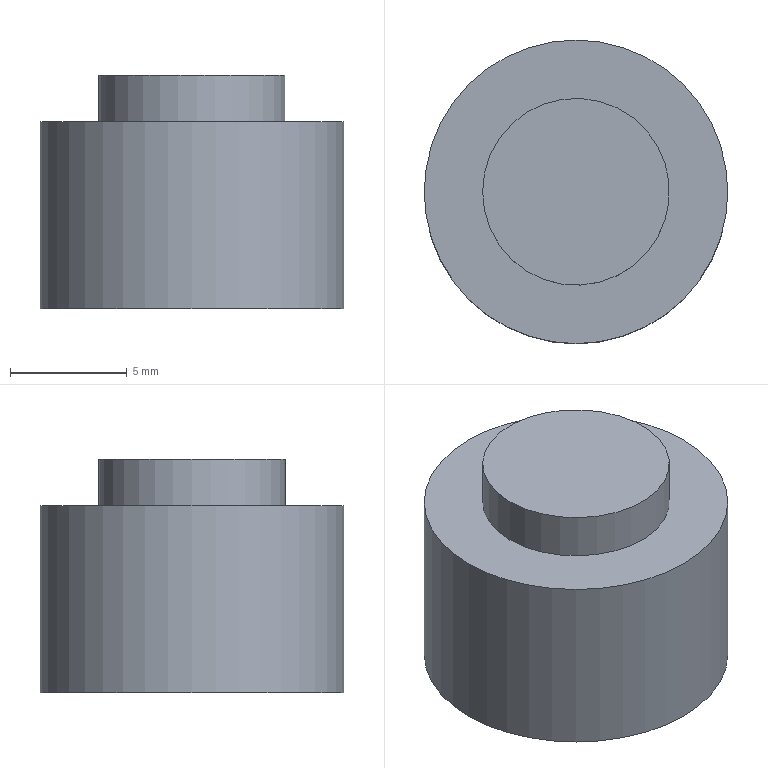Part | STEP file | gslz 2016.10.28-10_id574_x_t | 1 solid | 12 faces | box 13 x 13 x 10 mm | volume 1038 mm3 | plane 10 | cylinder 2 | commonest cylinder face diameters 8 x1 13 x1
STEP:
#1=CARTESIAN_POINT('',(0.,0.,0.));
#2=DIRECTION('',(0.,0.,1.));
#3=DIRECTION('',(1.,0.,0.));
#4=AXIS2_PLACEMENT_3D('',#1,#2,#3);
#5=CARTESIAN_POINT('',(-232.7,210.,99.));
#6=VERTEX_POINT('',#5);
#7=CARTESIAN_POINT('',(-228.7,210.,99.));
#8=DIRECTION('',(0.,0.,1.));
#9=DIRECTION('',(-1.,0.,0.));
#10=AXIS2_PLACEMENT_3D('',#7,#8,#9);
#11=CIRCLE('',#10,4.);
#12=CARTESIAN_POINT('',(-228.7,210.,99.));
#13=DIRECTION('',(0.,0.,1.));
#14=DIRECTION('',(1.,0.,0.));
#15=AXIS2_PLACEMENT_3D('',#12,#13,#14);
#16=PLANE('',#15);
#17=CARTESIAN_POINT('',(0.,0.));
#18=DIRECTION('',(-1.,0.));
#19=AXIS2_PLACEMENT_2D('',#17,#18);
#20=CIRCLE('',#19,4.);
#21=(GEOMETRIC_REPRESENTATION_CONTEXT(2)PARAMETRIC_REPRESENTATION_CONTEXT()REPRESENTATION_CONTEXT('',''));
#22=DEFINITIONAL_REPRESENTATION('',(#20),#21);
#23=PCURVE('',#16,#22);
#24=CARTESIAN_POINT('',(-228.7,210.,88.));
#25=DIRECTION('',(0.,0.,1.));
#26=DIRECTION('',(1.,0.,0.));
#27=AXIS2_PLACEMENT_3D('',#24,#25,#26);
#28=CYLINDRICAL_SURFACE('',#27,4.);
#29=CARTESIAN_POINT('',(3.142,11.));
#30=DIRECTION('',(1.,0.));
#31=VECTOR('',#30,1.);
#32=LINE('',#29,#31);
#33=(GEOMETRIC_REPRESENTATION_CONTEXT(2)PARAMETRIC_REPRESENTATION_CONTEXT()REPRESENTATION_CONTEXT('',''));
#34=DEFINITIONAL_REPRESENTATION('',(#32),#33);
#35=PCURVE('',#28,#34);
#36=SURFACE_CURVE('',#11,(#23,#35),.PCURVE_S1.);
#37=EDGE_CURVE('',#6,#6,#36,.T.);
#38=ORIENTED_EDGE('',*,*,#37,.T.);
#39=EDGE_LOOP('',(#38));
#40=FACE_BOUND('',#39,.T.);
#41=ADVANCED_FACE('',(#40),#16,.T.);
#42=CARTESIAN_POINT('',(-228.7,213.46,93.));
#43=VERTEX_POINT('',#42);
#44=CARTESIAN_POINT('',(-225.7,211.728,93.));
#45=VERTEX_POINT('',#44);
#46=CARTESIAN_POINT('',(-227.2,212.594,93.));
#47=DIRECTION('',(0.866,-0.5,0.));
#48=VECTOR('',#47,1.);
#49=LINE('',#46,#48);
#50=CARTESIAN_POINT('',(-228.7,209.995,93.));
#51=DIRECTION('',(0.,0.,1.));
#52=DIRECTION('',(1.,0.,0.));
#53=AXIS2_PLACEMENT_3D('',#50,#51,#52);
#54=PLANE('',#53);
#55=CARTESIAN_POINT('',(1.5,2.599));
#56=DIRECTION('',(0.866,-0.5));
#57=VECTOR('',#56,1.);
#58=LINE('',#55,#57);
#59=(GEOMETRIC_REPRESENTATION_CONTEXT(2)PARAMETRIC_REPRESENTATION_CONTEXT()REPRESENTATION_CONTEXT('',''));
#60=DEFINITIONAL_REPRESENTATION('',(#58),#59);
#61=PCURVE('',#54,#60);
#62=CARTESIAN_POINT('',(-228.7,213.46,93.));
#63=DIRECTION('',(-0.5,-0.866,0.));
#64=DIRECTION('',(0.866,-0.5,0.));
#65=AXIS2_PLACEMENT_3D('',#62,#63,#64);
#66=PLANE('',#65);
#67=CARTESIAN_POINT('',(1.732,0.));
#68=DIRECTION('',(1.,0.));
#69=VECTOR('',#68,1.);
#70=LINE('',#67,#69);
#71=(GEOMETRIC_REPRESENTATION_CONTEXT(2)PARAMETRIC_REPRESENTATION_CONTEXT()REPRESENTATION_CONTEXT('',''));
#72=DEFINITIONAL_REPRESENTATION('',(#70),#71);
#73=PCURVE('',#66,#72);
#74=SURFACE_CURVE('',#49,(#61,#73),.PCURVE_S1.);
#75=EDGE_CURVE('',#43,#45,#74,.T.);
#76=ORIENTED_EDGE('',*,*,#75,.T.);
#77=CARTESIAN_POINT('',(-225.7,208.262,93.));
#78=VERTEX_POINT('',#77);
#79=CARTESIAN_POINT('',(-225.7,209.995,93.));
#80=DIRECTION('',(0.,1.,0.));
#81=VECTOR('',#80,1.);
#82=LINE('',#79,#81);
#83=CARTESIAN_POINT('',(3.,0.));
#84=DIRECTION('',(0.,1.));
#85=VECTOR('',#84,1.);
#86=LINE('',#83,#85);
#87=(GEOMETRIC_REPRESENTATION_CONTEXT(2)PARAMETRIC_REPRESENTATION_CONTEXT()REPRESENTATION_CONTEXT('',''));
#88=DEFINITIONAL_REPRESENTATION('',(#86),#87);
#89=PCURVE('',#54,#88);
#90=CARTESIAN_POINT('',(-225.7,209.995,93.));
#91=DIRECTION('',(1.,0.,0.));
#92=DIRECTION('',(0.,0.,-1.));
#93=AXIS2_PLACEMENT_3D('',#90,#91,#92);
#94=PLANE('',#93);
#95=CARTESIAN_POINT('',(0.,0.));
#96=DIRECTION('',(0.,1.));
#97=VECTOR('',#96,1.);
#98=LINE('',#95,#97);
#99=(GEOMETRIC_REPRESENTATION_CONTEXT(2)PARAMETRIC_REPRESENTATION_CONTEXT()REPRESENTATION_CONTEXT('',''));
#100=DEFINITIONAL_REPRESENTATION('',(#98),#99);
#101=PCURVE('',#94,#100);
#102=SURFACE_CURVE('',#82,(#89,#101),.PCURVE_S1.);
#103=EDGE_CURVE('',#78,#45,#102,.T.);
#104=ORIENTED_EDGE('',*,*,#103,.F.);
#105=CARTESIAN_POINT('',(-228.7,206.53,93.));
#106=VERTEX_POINT('',#105);
#107=CARTESIAN_POINT('',(-227.2,207.396,93.));
#108=DIRECTION('',(-0.866,-0.5,0.));
#109=VECTOR('',#108,1.);
#110=LINE('',#107,#109);
#111=CARTESIAN_POINT('',(1.5,-2.599));
#112=DIRECTION('',(-0.866,-0.5));
#113=VECTOR('',#112,1.);
#114=LINE('',#111,#113);
#115=(GEOMETRIC_REPRESENTATION_CONTEXT(2)PARAMETRIC_REPRESENTATION_CONTEXT()REPRESENTATION_CONTEXT('',''));
#116=DEFINITIONAL_REPRESENTATION('',(#114),#115);
#117=PCURVE('',#54,#116);
#118=CARTESIAN_POINT('',(-225.7,208.262,93.));
#119=DIRECTION('',(-0.5,0.866,0.));
#120=DIRECTION('',(-0.866,-0.5,0.));
#121=AXIS2_PLACEMENT_3D('',#118,#119,#120);
#122=PLANE('',#121);
#123=CARTESIAN_POINT('',(1.732,0.));
#124=DIRECTION('',(1.,0.));
#125=VECTOR('',#124,1.);
#126=LINE('',#123,#125);
#127=(GEOMETRIC_REPRESENTATION_CONTEXT(2)PARAMETRIC_REPRESENTATION_CONTEXT()REPRESENTATION_CONTEXT('',''));
#128=DEFINITIONAL_REPRESENTATION('',(#126),#127);
#129=PCURVE('',#122,#128);
#130=SURFACE_CURVE('',#110,(#117,#129),.PCURVE_S1.);
#131=EDGE_CURVE('',#78,#106,#130,.T.);
#132=ORIENTED_EDGE('',*,*,#131,.T.);
#133=CARTESIAN_POINT('',(-231.7,208.262,93.));
#134=VERTEX_POINT('',#133);
#135=CARTESIAN_POINT('',(-230.2,207.396,93.));
#136=DIRECTION('',(-0.866,0.5,0.));
#137=VECTOR('',#136,1.);
#138=LINE('',#135,#137);
#139=CARTESIAN_POINT('',(-1.5,-2.599));
#140=DIRECTION('',(-0.866,0.5));
#141=VECTOR('',#140,1.);
#142=LINE('',#139,#141);
#143=(GEOMETRIC_REPRESENTATION_CONTEXT(2)PARAMETRIC_REPRESENTATION_CONTEXT()REPRESENTATION_CONTEXT('',''));
#144=DEFINITIONAL_REPRESENTATION('',(#142),#143);
#145=PCURVE('',#54,#144);
#146=CARTESIAN_POINT('',(-228.7,206.53,93.));
#147=DIRECTION('',(0.5,0.866,0.));
#148=DIRECTION('',(-0.866,0.5,0.));
#149=AXIS2_PLACEMENT_3D('',#146,#147,#148);
#150=PLANE('',#149);
#151=CARTESIAN_POINT('',(1.732,0.));
#152=DIRECTION('',(1.,0.));
#153=VECTOR('',#152,1.);
#154=LINE('',#151,#153);
#155=(GEOMETRIC_REPRESENTATION_CONTEXT(2)PARAMETRIC_REPRESENTATION_CONTEXT()REPRESENTATION_CONTEXT('',''));
#156=DEFINITIONAL_REPRESENTATION('',(#154),#155);
#157=PCURVE('',#150,#156);
#158=SURFACE_CURVE('',#138,(#145,#157),.PCURVE_S1.);
#159=EDGE_CURVE('',#106,#134,#158,.T.);
#160=ORIENTED_EDGE('',*,*,#159,.T.);
#161=CARTESIAN_POINT('',(-231.7,211.728,93.));
#162=VERTEX_POINT('',#161);
#163=CARTESIAN_POINT('',(-231.7,209.995,93.));
#164=DIRECTION('',(0.,-1.,0.));
#165=VECTOR('',#164,1.);
#166=LINE('',#163,#165);
#167=CARTESIAN_POINT('',(-3.,0.));
#168=DIRECTION('',(0.,-1.));
#169=VECTOR('',#168,1.);
#170=LINE('',#167,#169);
#171=(GEOMETRIC_REPRESENTATION_CONTEXT(2)PARAMETRIC_REPRESENTATION_CONTEXT()REPRESENTATION_CONTEXT('',''));
#172=DEFINITIONAL_REPRESENTATION('',(#170),#171);
#173=PCURVE('',#54,#172);
#174=CARTESIAN_POINT('',(-231.7,209.995,93.));
#175=DIRECTION('',(-1.,0.,0.));
#176=DIRECTION('',(0.,0.,1.));
#177=AXIS2_PLACEMENT_3D('',#174,#175,#176);
#178=PLANE('',#177);
#179=CARTESIAN_POINT('',(0.,0.));
#180=DIRECTION('',(0.,-1.));
#181=VECTOR('',#180,1.);
#182=LINE('',#179,#181);
#183=(GEOMETRIC_REPRESENTATION_CONTEXT(2)PARAMETRIC_REPRESENTATION_CONTEXT()REPRESENTATION_CONTEXT('',''));
#184=DEFINITIONAL_REPRESENTATION('',(#182),#183);
#185=PCURVE('',#178,#184);
#186=SURFACE_CURVE('',#166,(#173,#185),.PCURVE_S1.);
#187=EDGE_CURVE('',#162,#134,#186,.T.);
#188=ORIENTED_EDGE('',*,*,#187,.F.);
#189=CARTESIAN_POINT('',(-230.2,212.594,93.));
#190=DIRECTION('',(0.866,0.5,0.));
#191=VECTOR('',#190,1.);
#192=LINE('',#189,#191);
#193=CARTESIAN_POINT('',(-1.5,2.599));
#194=DIRECTION('',(0.866,0.5));
#195=VECTOR('',#194,1.);
#196=LINE('',#193,#195);
#197=(GEOMETRIC_REPRESENTATION_CONTEXT(2)PARAMETRIC_REPRESENTATION_CONTEXT()REPRESENTATION_CONTEXT('',''));
#198=DEFINITIONAL_REPRESENTATION('',(#196),#197);
#199=PCURVE('',#54,#198);
#200=CARTESIAN_POINT('',(-231.7,211.728,93.));
#201=DIRECTION('',(0.5,-0.866,0.));
#202=DIRECTION('',(0.866,0.5,0.));
#203=AXIS2_PLACEMENT_3D('',#200,#201,#202);
#204=PLANE('',#203);
#205=CARTESIAN_POINT('',(1.732,0.));
#206=DIRECTION('',(1.,0.));
#207=VECTOR('',#206,1.);
#208=LINE('',#205,#207);
#209=(GEOMETRIC_REPRESENTATION_CONTEXT(2)PARAMETRIC_REPRESENTATION_CONTEXT()REPRESENTATION_CONTEXT('',''));
#210=DEFINITIONAL_REPRESENTATION('',(#208),#209);
#211=PCURVE('',#204,#210);
#212=SURFACE_CURVE('',#192,(#199,#211),.PCURVE_S1.);
#213=EDGE_CURVE('',#162,#43,#212,.T.);
#214=ORIENTED_EDGE('',*,*,#213,.T.);
#215=EDGE_LOOP('',(#76,#104,#132,#160,#188,#214));
#216=FACE_BOUND('',#215,.T.);
#217=ADVANCED_FACE('',(#216),#54,.F.);
#218=ORIENTED_EDGE('',*,*,#187,.T.);
#219=CARTESIAN_POINT('',(-231.7,208.262,89.));
#220=VERTEX_POINT('',#219);
#221=CARTESIAN_POINT('',(-231.7,208.262,93.));
#222=DIRECTION('',(0.,0.,-1.));
#223=VECTOR('',#222,1.);
#224=LINE('',#221,#223);
#225=CARTESIAN_POINT('',(0.,-1.733));
#226=DIRECTION('',(-1.,0.));
#227=VECTOR('',#226,1.);
#228=LINE('',#225,#227);
#229=(GEOMETRIC_REPRESENTATION_CONTEXT(2)PARAMETRIC_REPRESENTATION_CONTEXT()REPRESENTATION_CONTEXT('',''));
#230=DEFINITIONAL_REPRESENTATION('',(#228),#229);
#231=PCURVE('',#178,#230);
#232=CARTESIAN_POINT('',(3.464,0.));
#233=DIRECTION('',(0.,-1.));
#234=VECTOR('',#233,1.);
#235=LINE('',#232,#234);
#236=(GEOMETRIC_REPRESENTATION_CONTEXT(2)PARAMETRIC_REPRESENTATION_CONTEXT()REPRESENTATION_CONTEXT('',''));
#237=DEFINITIONAL_REPRESENTATION('',(#235),#236);
#238=PCURVE('',#150,#237);
#239=SURFACE_CURVE('',#224,(#231,#238),.PCURVE_S1.);
#240=EDGE_CURVE('',#134,#220,#239,.T.);
#241=ORIENTED_EDGE('',*,*,#240,.T.);
#242=CARTESIAN_POINT('',(-231.7,211.728,89.));
#243=VERTEX_POINT('',#242);
#244=CARTESIAN_POINT('',(-231.7,209.995,89.));
#245=DIRECTION('',(0.,-1.,0.));
#246=VECTOR('',#245,1.);
#247=LINE('',#244,#246);
#248=CARTESIAN_POINT('',(-4.,0.));
#249=DIRECTION('',(0.,-1.));
#250=VECTOR('',#249,1.);
#251=LINE('',#248,#250);
#252=(GEOMETRIC_REPRESENTATION_CONTEXT(2)PARAMETRIC_REPRESENTATION_CONTEXT()REPRESENTATION_CONTEXT('',''));
#253=DEFINITIONAL_REPRESENTATION('',(#251),#252);
#254=PCURVE('',#178,#253);
#255=CARTESIAN_POINT('',(-228.7,210.,89.));
#256=DIRECTION('',(0.,0.,-1.));
#257=DIRECTION('',(-1.,0.,0.));
#258=AXIS2_PLACEMENT_3D('',#255,#256,#257);
#259=PLANE('',#258);
#260=CARTESIAN_POINT('',(3.,-0.005));
#261=DIRECTION('',(0.,-1.));
#262=VECTOR('',#261,1.);
#263=LINE('',#260,#262);
#264=(GEOMETRIC_REPRESENTATION_CONTEXT(2)PARAMETRIC_REPRESENTATION_CONTEXT()REPRESENTATION_CONTEXT('',''));
#265=DEFINITIONAL_REPRESENTATION('',(#263),#264);
#266=PCURVE('',#259,#265);
#267=SURFACE_CURVE('',#247,(#254,#266),.PCURVE_S1.);
#268=EDGE_CURVE('',#243,#220,#267,.T.);
#269=ORIENTED_EDGE('',*,*,#268,.F.);
#270=CARTESIAN_POINT('',(-231.7,211.728,93.));
#271=DIRECTION('',(0.,0.,1.));
#272=VECTOR('',#271,1.);
#273=LINE('',#270,#272);
#274=CARTESIAN_POINT('',(0.,1.733));
#275=DIRECTION('',(1.,0.));
#276=VECTOR('',#275,1.);
#277=LINE('',#274,#276);
#278=(GEOMETRIC_REPRESENTATION_CONTEXT(2)PARAMETRIC_REPRESENTATION_CONTEXT()REPRESENTATION_CONTEXT('',''));
#279=DEFINITIONAL_REPRESENTATION('',(#277),#278);
#280=PCURVE('',#178,#279);
#281=CARTESIAN_POINT('',(0.,0.));
#282=DIRECTION('',(0.,1.));
#283=VECTOR('',#282,1.);
#284=LINE('',#281,#283);
#285=(GEOMETRIC_REPRESENTATION_CONTEXT(2)PARAMETRIC_REPRESENTATION_CONTEXT()REPRESENTATION_CONTEXT('',''));
#286=DEFINITIONAL_REPRESENTATION('',(#284),#285);
#287=PCURVE('',#204,#286);
#288=SURFACE_CURVE('',#273,(#280,#287),.PCURVE_S1.);
#289=EDGE_CURVE('',#243,#162,#288,.T.);
#290=ORIENTED_EDGE('',*,*,#289,.T.);
#291=EDGE_LOOP('',(#218,#241,#269,#290));
#292=FACE_BOUND('',#291,.T.);
#293=ADVANCED_FACE('',(#292),#178,.F.);
#294=ORIENTED_EDGE('',*,*,#213,.F.);
#295=ORIENTED_EDGE('',*,*,#289,.F.);
#296=CARTESIAN_POINT('',(-228.7,213.46,89.));
#297=VERTEX_POINT('',#296);
#298=CARTESIAN_POINT('',(-230.2,212.594,89.));
#299=DIRECTION('',(0.866,0.5,0.));
#300=VECTOR('',#299,1.);
#301=LINE('',#298,#300);
#302=CARTESIAN_POINT('',(1.732,-4.));
#303=DIRECTION('',(1.,0.));
#304=VECTOR('',#303,1.);
#305=LINE('',#302,#304);
#306=(GEOMETRIC_REPRESENTATION_CONTEXT(2)PARAMETRIC_REPRESENTATION_CONTEXT()REPRESENTATION_CONTEXT('',''));
#307=DEFINITIONAL_REPRESENTATION('',(#305),#306);
#308=PCURVE('',#204,#307);
#309=CARTESIAN_POINT('',(1.5,2.594));
#310=DIRECTION('',(-0.866,0.5));
#311=VECTOR('',#310,1.);
#312=LINE('',#309,#311);
#313=(GEOMETRIC_REPRESENTATION_CONTEXT(2)PARAMETRIC_REPRESENTATION_CONTEXT()REPRESENTATION_CONTEXT('',''));
#314=DEFINITIONAL_REPRESENTATION('',(#312),#313);
#315=PCURVE('',#259,#314);
#316=SURFACE_CURVE('',#301,(#308,#315),.PCURVE_S1.);
#317=EDGE_CURVE('',#243,#297,#316,.T.);
#318=ORIENTED_EDGE('',*,*,#317,.T.);
#319=CARTESIAN_POINT('',(-228.7,213.46,93.));
#320=DIRECTION('',(0.,0.,1.));
#321=VECTOR('',#320,1.);
#322=LINE('',#319,#321);
#323=CARTESIAN_POINT('',(3.464,0.));
#324=DIRECTION('',(0.,1.));
#325=VECTOR('',#324,1.);
#326=LINE('',#323,#325);
#327=(GEOMETRIC_REPRESENTATION_CONTEXT(2)PARAMETRIC_REPRESENTATION_CONTEXT()REPRESENTATION_CONTEXT('',''));
#328=DEFINITIONAL_REPRESENTATION('',(#326),#327);
#329=PCURVE('',#204,#328);
#330=CARTESIAN_POINT('',(0.,0.));
#331=DIRECTION('',(0.,1.));
#332=VECTOR('',#331,1.);
#333=LINE('',#330,#332);
#334=(GEOMETRIC_REPRESENTATION_CONTEXT(2)PARAMETRIC_REPRESENTATION_CONTEXT()REPRESENTATION_CONTEXT('',''));
#335=DEFINITIONAL_REPRESENTATION('',(#333),#334);
#336=PCURVE('',#66,#335);
#337=SURFACE_CURVE('',#322,(#329,#336),.PCURVE_S1.);
#338=EDGE_CURVE('',#297,#43,#337,.T.);
#339=ORIENTED_EDGE('',*,*,#338,.T.);
#340=EDGE_LOOP('',(#294,#295,#318,#339));
#341=FACE_BOUND('',#340,.T.);
#342=ADVANCED_FACE('',(#341),#204,.T.);
#343=ORIENTED_EDGE('',*,*,#75,.F.);
#344=ORIENTED_EDGE('',*,*,#338,.F.);
#345=CARTESIAN_POINT('',(-225.7,211.728,89.));
#346=VERTEX_POINT('',#345);
#347=CARTESIAN_POINT('',(-227.2,212.594,89.));
#348=DIRECTION('',(0.866,-0.5,0.));
#349=VECTOR('',#348,1.);
#350=LINE('',#347,#349);
#351=CARTESIAN_POINT('',(1.732,-4.));
#352=DIRECTION('',(1.,0.));
#353=VECTOR('',#352,1.);
#354=LINE('',#351,#353);
#355=(GEOMETRIC_REPRESENTATION_CONTEXT(2)PARAMETRIC_REPRESENTATION_CONTEXT()REPRESENTATION_CONTEXT('',''));
#356=DEFINITIONAL_REPRESENTATION('',(#354),#355);
#357=PCURVE('',#66,#356);
#358=CARTESIAN_POINT('',(-1.5,2.594));
#359=DIRECTION('',(-0.866,-0.5));
#360=VECTOR('',#359,1.);
#361=LINE('',#358,#360);
#362=(GEOMETRIC_REPRESENTATION_CONTEXT(2)PARAMETRIC_REPRESENTATION_CONTEXT()REPRESENTATION_CONTEXT('',''));
#363=DEFINITIONAL_REPRESENTATION('',(#361),#362);
#364=PCURVE('',#259,#363);
#365=SURFACE_CURVE('',#350,(#357,#364),.PCURVE_S1.);
#366=EDGE_CURVE('',#297,#346,#365,.T.);
#367=ORIENTED_EDGE('',*,*,#366,.T.);
#368=CARTESIAN_POINT('',(-225.7,211.728,93.));
#369=DIRECTION('',(0.,0.,-1.));
#370=VECTOR('',#369,1.);
#371=LINE('',#368,#370);
#372=CARTESIAN_POINT('',(3.464,0.));
#373=DIRECTION('',(0.,-1.));
#374=VECTOR('',#373,1.);
#375=LINE('',#372,#374);
#376=(GEOMETRIC_REPRESENTATION_CONTEXT(2)PARAMETRIC_REPRESENTATION_CONTEXT()REPRESENTATION_CONTEXT('',''));
#377=DEFINITIONAL_REPRESENTATION('',(#375),#376);
#378=PCURVE('',#66,#377);
#379=CARTESIAN_POINT('',(0.,1.733));
#380=DIRECTION('',(1.,0.));
#381=VECTOR('',#380,1.);
#382=LINE('',#379,#381);
#383=(GEOMETRIC_REPRESENTATION_CONTEXT(2)PARAMETRIC_REPRESENTATION_CONTEXT()REPRESENTATION_CONTEXT('',''));
#384=DEFINITIONAL_REPRESENTATION('',(#382),#383);
#385=PCURVE('',#94,#384);
#386=SURFACE_CURVE('',#371,(#378,#385),.PCURVE_S1.);
#387=EDGE_CURVE('',#45,#346,#386,.T.);
#388=ORIENTED_EDGE('',*,*,#387,.F.);
#389=EDGE_LOOP('',(#343,#344,#367,#388));
#390=FACE_BOUND('',#389,.T.);
#391=ADVANCED_FACE('',(#390),#66,.T.);
#392=CARTESIAN_POINT('',(-225.7,208.262,89.));
#393=VERTEX_POINT('',#392);
#394=CARTESIAN_POINT('',(-225.7,209.995,89.));
#395=DIRECTION('',(0.,1.,0.));
#396=VECTOR('',#395,1.);
#397=LINE('',#394,#396);
#398=CARTESIAN_POINT('',(4.,0.));
#399=DIRECTION('',(0.,1.));
#400=VECTOR('',#399,1.);
#401=LINE('',#398,#400);
#402=(GEOMETRIC_REPRESENTATION_CONTEXT(2)PARAMETRIC_REPRESENTATION_CONTEXT()REPRESENTATION_CONTEXT('',''));
#403=DEFINITIONAL_REPRESENTATION('',(#401),#402);
#404=PCURVE('',#94,#403);
#405=CARTESIAN_POINT('',(-3.,-0.005));
#406=DIRECTION('',(0.,1.));
#407=VECTOR('',#406,1.);
#408=LINE('',#405,#407);
#409=(GEOMETRIC_REPRESENTATION_CONTEXT(2)PARAMETRIC_REPRESENTATION_CONTEXT()REPRESENTATION_CONTEXT('',''));
#410=DEFINITIONAL_REPRESENTATION('',(#408),#409);
#411=PCURVE('',#259,#410);
#412=SURFACE_CURVE('',#397,(#404,#411),.PCURVE_S1.);
#413=EDGE_CURVE('',#393,#346,#412,.T.);
#414=ORIENTED_EDGE('',*,*,#413,.F.);
#415=CARTESIAN_POINT('',(-225.7,208.262,93.));
#416=DIRECTION('',(0.,0.,1.));
#417=VECTOR('',#416,1.);
#418=LINE('',#415,#417);
#419=CARTESIAN_POINT('',(0.,-1.733));
#420=DIRECTION('',(-1.,0.));
#421=VECTOR('',#420,1.);
#422=LINE('',#419,#421);
#423=(GEOMETRIC_REPRESENTATION_CONTEXT(2)PARAMETRIC_REPRESENTATION_CONTEXT()REPRESENTATION_CONTEXT('',''));
#424=DEFINITIONAL_REPRESENTATION('',(#422),#423);
#425=PCURVE('',#94,#424);
#426=CARTESIAN_POINT('',(0.,0.));
#427=DIRECTION('',(0.,1.));
#428=VECTOR('',#427,1.);
#429=LINE('',#426,#428);
#430=(GEOMETRIC_REPRESENTATION_CONTEXT(2)PARAMETRIC_REPRESENTATION_CONTEXT()REPRESENTATION_CONTEXT('',''));
#431=DEFINITIONAL_REPRESENTATION('',(#429),#430);
#432=PCURVE('',#122,#431);
#433=SURFACE_CURVE('',#418,(#425,#432),.PCURVE_S1.);
#434=EDGE_CURVE('',#393,#78,#433,.T.);
#435=ORIENTED_EDGE('',*,*,#434,.T.);
#436=ORIENTED_EDGE('',*,*,#103,.T.);
#437=ORIENTED_EDGE('',*,*,#387,.T.);
#438=EDGE_LOOP('',(#414,#435,#436,#437));
#439=FACE_BOUND('',#438,.T.);
#440=ADVANCED_FACE('',(#439),#94,.F.);
#441=ORIENTED_EDGE('',*,*,#131,.F.);
#442=ORIENTED_EDGE('',*,*,#434,.F.);
#443=CARTESIAN_POINT('',(-228.7,206.53,89.));
#444=VERTEX_POINT('',#443);
#445=CARTESIAN_POINT('',(-227.2,207.396,89.));
#446=DIRECTION('',(-0.866,-0.5,0.));
#447=VECTOR('',#446,1.);
#448=LINE('',#445,#447);
#449=CARTESIAN_POINT('',(1.732,-4.));
#450=DIRECTION('',(1.,0.));
#451=VECTOR('',#450,1.);
#452=LINE('',#449,#451);
#453=(GEOMETRIC_REPRESENTATION_CONTEXT(2)PARAMETRIC_REPRESENTATION_CONTEXT()REPRESENTATION_CONTEXT('',''));
#454=DEFINITIONAL_REPRESENTATION('',(#452),#453);
#455=PCURVE('',#122,#454);
#456=CARTESIAN_POINT('',(-1.5,-2.604));
#457=DIRECTION('',(0.866,-0.5));
#458=VECTOR('',#457,1.);
#459=LINE('',#456,#458);
#460=(GEOMETRIC_REPRESENTATION_CONTEXT(2)PARAMETRIC_REPRESENTATION_CONTEXT()REPRESENTATION_CONTEXT('',''));
#461=DEFINITIONAL_REPRESENTATION('',(#459),#460);
#462=PCURVE('',#259,#461);
#463=SURFACE_CURVE('',#448,(#455,#462),.PCURVE_S1.);
#464=EDGE_CURVE('',#393,#444,#463,.T.);
#465=ORIENTED_EDGE('',*,*,#464,.T.);
#466=CARTESIAN_POINT('',(-228.7,206.53,93.));
#467=DIRECTION('',(0.,0.,1.));
#468=VECTOR('',#467,1.);
#469=LINE('',#466,#468);
#470=CARTESIAN_POINT('',(3.464,0.));
#471=DIRECTION('',(0.,1.));
#472=VECTOR('',#471,1.);
#473=LINE('',#470,#472);
#474=(GEOMETRIC_REPRESENTATION_CONTEXT(2)PARAMETRIC_REPRESENTATION_CONTEXT()REPRESENTATION_CONTEXT('',''));
#475=DEFINITIONAL_REPRESENTATION('',(#473),#474);
#476=PCURVE('',#122,#475);
#477=CARTESIAN_POINT('',(0.,0.));
#478=DIRECTION('',(0.,1.));
#479=VECTOR('',#478,1.);
#480=LINE('',#477,#479);
#481=(GEOMETRIC_REPRESENTATION_CONTEXT(2)PARAMETRIC_REPRESENTATION_CONTEXT()REPRESENTATION_CONTEXT('',''));
#482=DEFINITIONAL_REPRESENTATION('',(#480),#481);
#483=PCURVE('',#150,#482);
#484=SURFACE_CURVE('',#469,(#476,#483),.PCURVE_S1.);
#485=EDGE_CURVE('',#444,#106,#484,.T.);
#486=ORIENTED_EDGE('',*,*,#485,.T.);
#487=EDGE_LOOP('',(#441,#442,#465,#486));
#488=FACE_BOUND('',#487,.T.);
#489=ADVANCED_FACE('',(#488),#122,.T.);
#490=ORIENTED_EDGE('',*,*,#159,.F.);
#491=ORIENTED_EDGE('',*,*,#485,.F.);
#492=CARTESIAN_POINT('',(-230.2,207.396,89.));
#493=DIRECTION('',(-0.866,0.5,0.));
#494=VECTOR('',#493,1.);
#495=LINE('',#492,#494);
#496=CARTESIAN_POINT('',(1.732,-4.));
#497=DIRECTION('',(1.,0.));
#498=VECTOR('',#497,1.);
#499=LINE('',#496,#498);
#500=(GEOMETRIC_REPRESENTATION_CONTEXT(2)PARAMETRIC_REPRESENTATION_CONTEXT()REPRESENTATION_CONTEXT('',''));
#501=DEFINITIONAL_REPRESENTATION('',(#499),#500);
#502=PCURVE('',#150,#501);
#503=CARTESIAN_POINT('',(1.5,-2.604));
#504=DIRECTION('',(0.866,0.5));
#505=VECTOR('',#504,1.);
#506=LINE('',#503,#505);
#507=(GEOMETRIC_REPRESENTATION_CONTEXT(2)PARAMETRIC_REPRESENTATION_CONTEXT()REPRESENTATION_CONTEXT('',''));
#508=DEFINITIONAL_REPRESENTATION('',(#506),#507);
#509=PCURVE('',#259,#508);
#510=SURFACE_CURVE('',#495,(#502,#509),.PCURVE_S1.);
#511=EDGE_CURVE('',#444,#220,#510,.T.);
#512=ORIENTED_EDGE('',*,*,#511,.T.);
#513=ORIENTED_EDGE('',*,*,#240,.F.);
#514=EDGE_LOOP('',(#490,#491,#512,#513));
#515=FACE_BOUND('',#514,.T.);
#516=ADVANCED_FACE('',(#515),#150,.T.);
#517=ORIENTED_EDGE('',*,*,#511,.F.);
#518=ORIENTED_EDGE('',*,*,#464,.F.);
#519=ORIENTED_EDGE('',*,*,#413,.T.);
#520=ORIENTED_EDGE('',*,*,#366,.F.);
#521=ORIENTED_EDGE('',*,*,#317,.F.);
#522=ORIENTED_EDGE('',*,*,#268,.T.);
#523=EDGE_LOOP('',(#517,#518,#519,#520,#521,#522));
#524=FACE_BOUND('',#523,.T.);
#525=CARTESIAN_POINT('',(-222.2,210.,89.));
#526=VERTEX_POINT('',#525);
#527=CARTESIAN_POINT('',(-228.7,210.,89.));
#528=DIRECTION('',(0.,0.,1.));
#529=DIRECTION('',(1.,0.,0.));
#530=AXIS2_PLACEMENT_3D('',#527,#528,#529);
#531=CIRCLE('',#530,6.5);
#532=CARTESIAN_POINT('',(-6.5,0.));
#533=CARTESIAN_POINT('',(-6.5,11.258));
#534=CARTESIAN_POINT('',(3.25,5.629));
#535=CARTESIAN_POINT('',(13.,0.));
#536=CARTESIAN_POINT('',(3.25,-5.629));
#537=CARTESIAN_POINT('',(-6.5,-11.258));
#538=CARTESIAN_POINT('',(-6.5,0.));
#539=(BOUNDED_CURVE()B_SPLINE_CURVE(2,(#532,#533,#534,#535,#536,#537,#538),.UNSPECIFIED.,.T.,.F.)B_SPLINE_CURVE_WITH_KNOTS((1,2,2,2,2,1),(-2.094,0.,2.094,4.189,6.283,8.378),.UNSPECIFIED.)CURVE()GEOMETRIC_REPRESENTATION_ITEM()RATIONAL_B_SPLINE_CURVE((1.,0.5,1.,0.5,1.,0.5,1.))REPRESENTATION_ITEM(''));
#540=(GEOMETRIC_REPRESENTATION_CONTEXT(2)PARAMETRIC_REPRESENTATION_CONTEXT()REPRESENTATION_CONTEXT('',''));
#541=DEFINITIONAL_REPRESENTATION('',(#539),#540);
#542=PCURVE('',#259,#541);
#543=CARTESIAN_POINT('',(-228.7,210.,88.));
#544=DIRECTION('',(0.,0.,1.));
#545=DIRECTION('',(1.,0.,0.));
#546=AXIS2_PLACEMENT_3D('',#543,#544,#545);
#547=CYLINDRICAL_SURFACE('',#546,6.5);
#548=CARTESIAN_POINT('',(0.,1.));
#549=DIRECTION('',(1.,0.));
#550=VECTOR('',#549,1.);
#551=LINE('',#548,#550);
#552=(GEOMETRIC_REPRESENTATION_CONTEXT(2)PARAMETRIC_REPRESENTATION_CONTEXT()REPRESENTATION_CONTEXT('',''));
#553=DEFINITIONAL_REPRESENTATION('',(#551),#552);
#554=PCURVE('',#547,#553);
#555=SURFACE_CURVE('',#531,(#542,#554),.PCURVE_S1.);
#556=EDGE_CURVE('',#526,#526,#555,.T.);
#557=ORIENTED_EDGE('',*,*,#556,.F.);
#558=EDGE_LOOP('',(#557));
#559=FACE_BOUND('',#558,.T.);
#560=ADVANCED_FACE('',(#524,#559),#259,.T.);
#561=CARTESIAN_POINT('',(-222.2,210.,97.));
#562=VERTEX_POINT('',#561);
#563=CARTESIAN_POINT('',(-228.7,210.,97.));
#564=DIRECTION('',(0.,0.,-1.));
#565=DIRECTION('',(1.,0.,0.));
#566=AXIS2_PLACEMENT_3D('',#563,#564,#565);
#567=CIRCLE('',#566,6.5);
#568=CARTESIAN_POINT('',(6.283,9.));
#569=DIRECTION('',(-1.,0.));
#570=VECTOR('',#569,1.);
#571=LINE('',#568,#570);
#572=(GEOMETRIC_REPRESENTATION_CONTEXT(2)PARAMETRIC_REPRESENTATION_CONTEXT()REPRESENTATION_CONTEXT('',''));
#573=DEFINITIONAL_REPRESENTATION('',(#571),#572);
#574=PCURVE('',#547,#573);
#575=CARTESIAN_POINT('',(-228.7,210.,97.));
#576=DIRECTION('',(0.,0.,1.));
#577=DIRECTION('',(1.,0.,0.));
#578=AXIS2_PLACEMENT_3D('',#575,#576,#577);
#579=PLANE('',#578);
#580=CARTESIAN_POINT('',(6.5,0.));
#581=CARTESIAN_POINT('',(6.5,-11.258));
#582=CARTESIAN_POINT('',(-3.25,-5.629));
#583=CARTESIAN_POINT('',(-13.,0.));
#584=CARTESIAN_POINT('',(-3.25,5.629));
#585=CARTESIAN_POINT('',(6.5,11.258));
#586=CARTESIAN_POINT('',(6.5,0.));
#587=(BOUNDED_CURVE()B_SPLINE_CURVE(2,(#580,#581,#582,#583,#584,#585,#586),.UNSPECIFIED.,.T.,.F.)B_SPLINE_CURVE_WITH_KNOTS((1,2,2,2,2,1),(-2.094,0.,2.094,4.189,6.283,8.378),.UNSPECIFIED.)CURVE()GEOMETRIC_REPRESENTATION_ITEM()RATIONAL_B_SPLINE_CURVE((1.,0.5,1.,0.5,1.,0.5,1.))REPRESENTATION_ITEM(''));
#588=(GEOMETRIC_REPRESENTATION_CONTEXT(2)PARAMETRIC_REPRESENTATION_CONTEXT()REPRESENTATION_CONTEXT('',''));
#589=DEFINITIONAL_REPRESENTATION('',(#587),#588);
#590=PCURVE('',#579,#589);
#591=SURFACE_CURVE('',#567,(#574,#590),.PCURVE_S1.);
#592=EDGE_CURVE('',#562,#562,#591,.T.);
#593=ORIENTED_EDGE('',*,*,#592,.T.);
#594=CARTESIAN_POINT('',(-222.2,210.,89.));
#595=CARTESIAN_POINT('',(-222.2,210.,97.));
#596=B_SPLINE_CURVE_WITH_KNOTS('',1,(#594,#595),.UNSPECIFIED.,.F.,.F.,(2,2),(1.,9.),.PIECEWISE_BEZIER_KNOTS.);
#597=CARTESIAN_POINT('',(0.,0.));
#598=DIRECTION('',(0.,1.));
#599=VECTOR('',#598,1.);
#600=LINE('',#597,#599);
#601=(GEOMETRIC_REPRESENTATION_CONTEXT(2)PARAMETRIC_REPRESENTATION_CONTEXT()REPRESENTATION_CONTEXT('',''));
#602=DEFINITIONAL_REPRESENTATION('',(#600),#601);
#603=PCURVE('',#547,#602);
#604=CARTESIAN_POINT('',(6.283,0.));
#605=DIRECTION('',(0.,1.));
#606=VECTOR('',#605,1.);
#607=LINE('',#604,#606);
#608=(GEOMETRIC_REPRESENTATION_CONTEXT(2)PARAMETRIC_REPRESENTATION_CONTEXT()REPRESENTATION_CONTEXT('',''));
#609=DEFINITIONAL_REPRESENTATION('',(#607),#608);
#610=PCURVE('',#547,#609);
#611=SEAM_CURVE('',#596,(#603,#610),.PCURVE_S1.);
#612=EDGE_CURVE('',#526,#562,#611,.T.);
#613=ORIENTED_EDGE('',*,*,#612,.F.);
#614=ORIENTED_EDGE('',*,*,#556,.T.);
#615=ORIENTED_EDGE('',*,*,#612,.T.);
#616=EDGE_LOOP('',(#593,#613,#614,#615));
#617=FACE_BOUND('',#616,.T.);
#618=ADVANCED_FACE('',(#617),#547,.T.);
#619=CARTESIAN_POINT('',(-232.7,210.,97.));
#620=VERTEX_POINT('',#619);
#621=CARTESIAN_POINT('',(-228.7,210.,97.));
#622=DIRECTION('',(0.,0.,1.));
#623=DIRECTION('',(-1.,0.,0.));
#624=AXIS2_PLACEMENT_3D('',#621,#622,#623);
#625=CIRCLE('',#624,4.);
#626=CARTESIAN_POINT('',(0.,0.));
#627=DIRECTION('',(-1.,0.));
#628=AXIS2_PLACEMENT_2D('',#626,#627);
#629=CIRCLE('',#628,4.);
#630=(GEOMETRIC_REPRESENTATION_CONTEXT(2)PARAMETRIC_REPRESENTATION_CONTEXT()REPRESENTATION_CONTEXT('',''));
#631=DEFINITIONAL_REPRESENTATION('',(#629),#630);
#632=PCURVE('',#579,#631);
#633=CARTESIAN_POINT('',(3.142,9.));
#634=DIRECTION('',(1.,0.));
#635=VECTOR('',#634,1.);
#636=LINE('',#633,#635);
#637=(GEOMETRIC_REPRESENTATION_CONTEXT(2)PARAMETRIC_REPRESENTATION_CONTEXT()REPRESENTATION_CONTEXT('',''));
#638=DEFINITIONAL_REPRESENTATION('',(#636),#637);
#639=PCURVE('',#28,#638);
#640=SURFACE_CURVE('',#625,(#632,#639),.PCURVE_S1.);
#641=EDGE_CURVE('',#620,#620,#640,.T.);
#642=ORIENTED_EDGE('',*,*,#641,.F.);
#643=EDGE_LOOP('',(#642));
#644=FACE_BOUND('',#643,.T.);
#645=ORIENTED_EDGE('',*,*,#592,.F.);
#646=EDGE_LOOP('',(#645));
#647=FACE_BOUND('',#646,.T.);
#648=ADVANCED_FACE('',(#644,#647),#579,.T.);
#649=ORIENTED_EDGE('',*,*,#641,.T.);
#650=CARTESIAN_POINT('',(-232.7,210.,97.));
#651=CARTESIAN_POINT('',(-232.7,210.,99.));
#652=B_SPLINE_CURVE_WITH_KNOTS('',1,(#650,#651),.UNSPECIFIED.,.F.,.F.,(2,2),(9.,11.),.PIECEWISE_BEZIER_KNOTS.);
#653=CARTESIAN_POINT('',(9.425,0.));
#654=DIRECTION('',(0.,1.));
#655=VECTOR('',#654,1.);
#656=LINE('',#653,#655);
#657=(GEOMETRIC_REPRESENTATION_CONTEXT(2)PARAMETRIC_REPRESENTATION_CONTEXT()REPRESENTATION_CONTEXT('',''));
#658=DEFINITIONAL_REPRESENTATION('',(#656),#657);
#659=PCURVE('',#28,#658);
#660=CARTESIAN_POINT('',(3.142,0.));
#661=DIRECTION('',(0.,1.));
#662=VECTOR('',#661,1.);
#663=LINE('',#660,#662);
#664=(GEOMETRIC_REPRESENTATION_CONTEXT(2)PARAMETRIC_REPRESENTATION_CONTEXT()REPRESENTATION_CONTEXT('',''));
#665=DEFINITIONAL_REPRESENTATION('',(#663),#664);
#666=PCURVE('',#28,#665);
#667=SEAM_CURVE('',#652,(#659,#666),.PCURVE_S1.);
#668=EDGE_CURVE('',#620,#6,#667,.T.);
#669=ORIENTED_EDGE('',*,*,#668,.T.);
#670=ORIENTED_EDGE('',*,*,#37,.F.);
#671=ORIENTED_EDGE('',*,*,#668,.F.);
#672=EDGE_LOOP('',(#649,#669,#670,#671));
#673=FACE_BOUND('',#672,.T.);
#674=ADVANCED_FACE('',(#673),#28,.T.);
#675=CLOSED_SHELL('',(#41,#217,#293,#342,#391,#440,#489,#516,#560,#618,#648,#674));
#676=MANIFOLD_SOLID_BREP('',#675);
#677=(LENGTH_UNIT()NAMED_UNIT(*)SI_UNIT(.MILLI.,.METRE.));
#678=UNCERTAINTY_MEASURE_WITH_UNIT(LENGTH_MEASURE(0.000002),#677,'','');
#679=(NAMED_UNIT(*)PLANE_ANGLE_UNIT()SI_UNIT($,.RADIAN.));
#680=(NAMED_UNIT(*)SI_UNIT($,.STERADIAN.)SOLID_ANGLE_UNIT());
#681=(GEOMETRIC_REPRESENTATION_CONTEXT(3)GLOBAL_UNCERTAINTY_ASSIGNED_CONTEXT((#678))GLOBAL_UNIT_ASSIGNED_CONTEXT((#677,#679,#680))REPRESENTATION_CONTEXT('',''));
#682=ADVANCED_BREP_SHAPE_REPRESENTATION('',(#4,#676),#681);